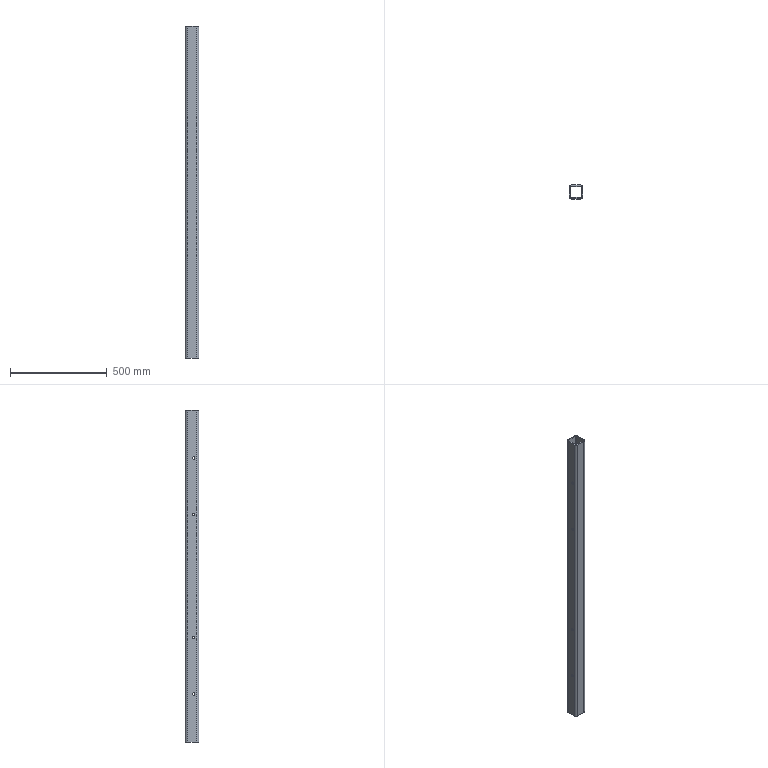Part | SolidWorks | features Extrusion 1, ICE 1, LPattern 1 | 1 solid | 34 faces | box 70 x 70 x 1716 mm | volume 2470318 mm3 | cylinder 24 | plane 10 | commonest cylinder face diameters 13 x16 12 x4 24 x4
STEP:
#1=CARTESIAN_POINT('',(70.,26.,1461.5));
#2=VERTEX_POINT('',#1);
#3=CARTESIAN_POINT('',(70.,26.,1474.5));
#4=VERTEX_POINT('',#3);
#5=CARTESIAN_POINT('',(70.,26.,1468.));
#6=DIRECTION('',(-1.,0.,0.));
#7=DIRECTION('',(0.,0.,1.));
#8=AXIS2_PLACEMENT_3D('',#5,#6,#7);
#9=CIRCLE('',#8,6.5);
#10=EDGE_CURVE('',#2,#4,#9,.T.);
#11=ORIENTED_EDGE('',*,*,#10,.F.);
#12=CARTESIAN_POINT('',(64.,26.,1461.5));
#13=VERTEX_POINT('',#12);
#14=CARTESIAN_POINT('',(70.,26.,1461.5));
#15=DIRECTION('',(-1.,0.,0.));
#16=VECTOR('',#15,1000.);
#17=LINE('',#14,#16);
#18=EDGE_CURVE('',#2,#13,#17,.T.);
#19=ORIENTED_EDGE('',*,*,#18,.T.);
#20=CARTESIAN_POINT('',(64.,26.,1474.5));
#21=VERTEX_POINT('',#20);
#22=CARTESIAN_POINT('',(64.,26.,1468.));
#23=DIRECTION('',(-1.,0.,0.));
#24=DIRECTION('',(0.,0.,1.));
#25=AXIS2_PLACEMENT_3D('',#22,#23,#24);
#26=CIRCLE('',#25,6.5);
#27=EDGE_CURVE('',#13,#21,#26,.T.);
#28=ORIENTED_EDGE('',*,*,#27,.T.);
#29=CARTESIAN_POINT('',(70.,26.,1474.5));
#30=DIRECTION('',(-1.,0.,0.));
#31=VECTOR('',#30,1000.);
#32=LINE('',#29,#31);
#33=EDGE_CURVE('',#4,#21,#32,.T.);
#34=ORIENTED_EDGE('',*,*,#33,.F.);
#35=EDGE_LOOP('',(#11,#19,#28,#34));
#36=FACE_OUTER_BOUND('',#35,.T.);
#37=CARTESIAN_POINT('',(70.,26.,1468.));
#38=DIRECTION('',(-1.,0.,0.));
#39=DIRECTION('',(0.,0.,1.));
#40=AXIS2_PLACEMENT_3D('',#37,#38,#39);
#41=CYLINDRICAL_SURFACE('',#40,6.5);
#42=ADVANCED_FACE('',(#36),#41,.F.);
#43=CARTESIAN_POINT('',(6.,26.,1474.5));
#44=VERTEX_POINT('',#43);
#45=CARTESIAN_POINT('',(6.,26.,1461.5));
#46=VERTEX_POINT('',#45);
#47=CARTESIAN_POINT('',(6.,26.,1468.));
#48=DIRECTION('',(1.,0.,0.));
#49=DIRECTION('',(0.,0.,-1.));
#50=AXIS2_PLACEMENT_3D('',#47,#48,#49);
#51=CIRCLE('',#50,6.5);
#52=EDGE_CURVE('',#44,#46,#51,.T.);
#53=ORIENTED_EDGE('',*,*,#52,.T.);
#54=CARTESIAN_POINT('',(0.,26.,1461.5));
#55=VERTEX_POINT('',#54);
#56=CARTESIAN_POINT('',(70.,26.,1461.5));
#57=DIRECTION('',(-1.,0.,0.));
#58=VECTOR('',#57,1000.);
#59=LINE('',#56,#58);
#60=EDGE_CURVE('',#46,#55,#59,.T.);
#61=ORIENTED_EDGE('',*,*,#60,.T.);
#62=CARTESIAN_POINT('',(0.,26.,1474.5));
#63=VERTEX_POINT('',#62);
#64=CARTESIAN_POINT('',(0.,26.,1468.));
#65=DIRECTION('',(-1.,0.,0.));
#66=DIRECTION('',(0.,0.,1.));
#67=AXIS2_PLACEMENT_3D('',#64,#65,#66);
#68=CIRCLE('',#67,6.5);
#69=EDGE_CURVE('',#55,#63,#68,.T.);
#70=ORIENTED_EDGE('',*,*,#69,.T.);
#71=CARTESIAN_POINT('',(70.,26.,1474.5));
#72=DIRECTION('',(-1.,0.,0.));
#73=VECTOR('',#72,1000.);
#74=LINE('',#71,#73);
#75=EDGE_CURVE('',#44,#63,#74,.T.);
#76=ORIENTED_EDGE('',*,*,#75,.F.);
#77=EDGE_LOOP('',(#53,#61,#70,#76));
#78=FACE_OUTER_BOUND('',#77,.T.);
#79=CARTESIAN_POINT('',(70.,26.,1468.));
#80=DIRECTION('',(-1.,0.,0.));
#81=DIRECTION('',(0.,0.,1.));
#82=AXIS2_PLACEMENT_3D('',#79,#80,#81);
#83=CYLINDRICAL_SURFACE('',#82,6.5);
#84=ADVANCED_FACE('',(#78),#83,.F.);
#85=CARTESIAN_POINT('',(70.,26.,1169.5));
#86=VERTEX_POINT('',#85);
#87=CARTESIAN_POINT('',(70.,26.,1182.5));
#88=VERTEX_POINT('',#87);
#89=CARTESIAN_POINT('',(70.,26.,1176.));
#90=DIRECTION('',(-1.,0.,0.));
#91=DIRECTION('',(0.,0.,1.));
#92=AXIS2_PLACEMENT_3D('',#89,#90,#91);
#93=CIRCLE('',#92,6.5);
#94=EDGE_CURVE('',#86,#88,#93,.T.);
#95=ORIENTED_EDGE('',*,*,#94,.F.);
#96=CARTESIAN_POINT('',(64.,26.,1169.5));
#97=VERTEX_POINT('',#96);
#98=CARTESIAN_POINT('',(70.,26.,1169.5));
#99=DIRECTION('',(-1.,0.,0.));
#100=VECTOR('',#99,1000.);
#101=LINE('',#98,#100);
#102=EDGE_CURVE('',#86,#97,#101,.T.);
#103=ORIENTED_EDGE('',*,*,#102,.T.);
#104=CARTESIAN_POINT('',(64.,26.,1182.5));
#105=VERTEX_POINT('',#104);
#106=CARTESIAN_POINT('',(64.,26.,1176.));
#107=DIRECTION('',(-1.,0.,0.));
#108=DIRECTION('',(0.,0.,1.));
#109=AXIS2_PLACEMENT_3D('',#106,#107,#108);
#110=CIRCLE('',#109,6.5);
#111=EDGE_CURVE('',#97,#105,#110,.T.);
#112=ORIENTED_EDGE('',*,*,#111,.T.);
#113=CARTESIAN_POINT('',(70.,26.,1182.5));
#114=DIRECTION('',(-1.,0.,0.));
#115=VECTOR('',#114,1000.);
#116=LINE('',#113,#115);
#117=EDGE_CURVE('',#88,#105,#116,.T.);
#118=ORIENTED_EDGE('',*,*,#117,.F.);
#119=EDGE_LOOP('',(#95,#103,#112,#118));
#120=FACE_OUTER_BOUND('',#119,.T.);
#121=CARTESIAN_POINT('',(70.,26.,1176.));
#122=DIRECTION('',(-1.,0.,0.));
#123=DIRECTION('',(0.,0.,1.));
#124=AXIS2_PLACEMENT_3D('',#121,#122,#123);
#125=CYLINDRICAL_SURFACE('',#124,6.5);
#126=ADVANCED_FACE('',(#120),#125,.F.);
#127=CARTESIAN_POINT('',(6.,26.,1182.5));
#128=VERTEX_POINT('',#127);
#129=CARTESIAN_POINT('',(6.,26.,1169.5));
#130=VERTEX_POINT('',#129);
#131=CARTESIAN_POINT('',(6.,26.,1176.));
#132=DIRECTION('',(1.,0.,0.));
#133=DIRECTION('',(0.,0.,-1.));
#134=AXIS2_PLACEMENT_3D('',#131,#132,#133);
#135=CIRCLE('',#134,6.5);
#136=EDGE_CURVE('',#128,#130,#135,.T.);
#137=ORIENTED_EDGE('',*,*,#136,.T.);
#138=CARTESIAN_POINT('',(0.,26.,1169.5));
#139=VERTEX_POINT('',#138);
#140=CARTESIAN_POINT('',(70.,26.,1169.5));
#141=DIRECTION('',(-1.,0.,0.));
#142=VECTOR('',#141,1000.);
#143=LINE('',#140,#142);
#144=EDGE_CURVE('',#130,#139,#143,.T.);
#145=ORIENTED_EDGE('',*,*,#144,.T.);
#146=CARTESIAN_POINT('',(0.,26.,1182.5));
#147=VERTEX_POINT('',#146);
#148=CARTESIAN_POINT('',(0.,26.,1176.));
#149=DIRECTION('',(-1.,0.,0.));
#150=DIRECTION('',(0.,0.,1.));
#151=AXIS2_PLACEMENT_3D('',#148,#149,#150);
#152=CIRCLE('',#151,6.5);
#153=EDGE_CURVE('',#139,#147,#152,.T.);
#154=ORIENTED_EDGE('',*,*,#153,.T.);
#155=CARTESIAN_POINT('',(70.,26.,1182.5));
#156=DIRECTION('',(-1.,0.,0.));
#157=VECTOR('',#156,1000.);
#158=LINE('',#155,#157);
#159=EDGE_CURVE('',#128,#147,#158,.T.);
#160=ORIENTED_EDGE('',*,*,#159,.F.);
#161=EDGE_LOOP('',(#137,#145,#154,#160));
#162=FACE_OUTER_BOUND('',#161,.T.);
#163=CARTESIAN_POINT('',(70.,26.,1176.));
#164=DIRECTION('',(-1.,0.,0.));
#165=DIRECTION('',(0.,0.,1.));
#166=AXIS2_PLACEMENT_3D('',#163,#164,#165);
#167=CYLINDRICAL_SURFACE('',#166,6.5);
#168=ADVANCED_FACE('',(#162),#167,.F.);
#169=CARTESIAN_POINT('',(70.,26.,533.5));
#170=VERTEX_POINT('',#169);
#171=CARTESIAN_POINT('',(70.,26.,546.5));
#172=VERTEX_POINT('',#171);
#173=CARTESIAN_POINT('',(70.,26.,540.));
#174=DIRECTION('',(-1.,0.,0.));
#175=DIRECTION('',(0.,0.,1.));
#176=AXIS2_PLACEMENT_3D('',#173,#174,#175);
#177=CIRCLE('',#176,6.5);
#178=EDGE_CURVE('',#170,#172,#177,.T.);
#179=ORIENTED_EDGE('',*,*,#178,.F.);
#180=CARTESIAN_POINT('',(64.,26.,533.5));
#181=VERTEX_POINT('',#180);
#182=CARTESIAN_POINT('',(70.,26.,533.5));
#183=DIRECTION('',(-1.,0.,0.));
#184=VECTOR('',#183,1000.);
#185=LINE('',#182,#184);
#186=EDGE_CURVE('',#170,#181,#185,.T.);
#187=ORIENTED_EDGE('',*,*,#186,.T.);
#188=CARTESIAN_POINT('',(64.,26.,546.5));
#189=VERTEX_POINT('',#188);
#190=CARTESIAN_POINT('',(64.,26.,540.));
#191=DIRECTION('',(-1.,0.,0.));
#192=DIRECTION('',(0.,0.,1.));
#193=AXIS2_PLACEMENT_3D('',#190,#191,#192);
#194=CIRCLE('',#193,6.5);
#195=EDGE_CURVE('',#181,#189,#194,.T.);
#196=ORIENTED_EDGE('',*,*,#195,.T.);
#197=CARTESIAN_POINT('',(70.,26.,546.5));
#198=DIRECTION('',(-1.,0.,0.));
#199=VECTOR('',#198,1000.);
#200=LINE('',#197,#199);
#201=EDGE_CURVE('',#172,#189,#200,.T.);
#202=ORIENTED_EDGE('',*,*,#201,.F.);
#203=EDGE_LOOP('',(#179,#187,#196,#202));
#204=FACE_OUTER_BOUND('',#203,.T.);
#205=CARTESIAN_POINT('',(70.,26.,540.));
#206=DIRECTION('',(-1.,0.,0.));
#207=DIRECTION('',(0.,0.,1.));
#208=AXIS2_PLACEMENT_3D('',#205,#206,#207);
#209=CYLINDRICAL_SURFACE('',#208,6.5);
#210=ADVANCED_FACE('',(#204),#209,.F.);
#211=CARTESIAN_POINT('',(6.,26.,546.5));
#212=VERTEX_POINT('',#211);
#213=CARTESIAN_POINT('',(6.,26.,533.5));
#214=VERTEX_POINT('',#213);
#215=CARTESIAN_POINT('',(6.,26.,540.));
#216=DIRECTION('',(1.,0.,0.));
#217=DIRECTION('',(0.,0.,-1.));
#218=AXIS2_PLACEMENT_3D('',#215,#216,#217);
#219=CIRCLE('',#218,6.5);
#220=EDGE_CURVE('',#212,#214,#219,.T.);
#221=ORIENTED_EDGE('',*,*,#220,.T.);
#222=CARTESIAN_POINT('',(0.,26.,533.5));
#223=VERTEX_POINT('',#222);
#224=CARTESIAN_POINT('',(70.,26.,533.5));
#225=DIRECTION('',(-1.,0.,0.));
#226=VECTOR('',#225,1000.);
#227=LINE('',#224,#226);
#228=EDGE_CURVE('',#214,#223,#227,.T.);
#229=ORIENTED_EDGE('',*,*,#228,.T.);
#230=CARTESIAN_POINT('',(0.,26.,546.5));
#231=VERTEX_POINT('',#230);
#232=CARTESIAN_POINT('',(0.,26.,540.));
#233=DIRECTION('',(-1.,0.,0.));
#234=DIRECTION('',(0.,0.,1.));
#235=AXIS2_PLACEMENT_3D('',#232,#233,#234);
#236=CIRCLE('',#235,6.5);
#237=EDGE_CURVE('',#223,#231,#236,.T.);
#238=ORIENTED_EDGE('',*,*,#237,.T.);
#239=CARTESIAN_POINT('',(70.,26.,546.5));
#240=DIRECTION('',(-1.,0.,0.));
#241=VECTOR('',#240,1000.);
#242=LINE('',#239,#241);
#243=EDGE_CURVE('',#212,#231,#242,.T.);
#244=ORIENTED_EDGE('',*,*,#243,.F.);
#245=EDGE_LOOP('',(#221,#229,#238,#244));
#246=FACE_OUTER_BOUND('',#245,.T.);
#247=CARTESIAN_POINT('',(70.,26.,540.));
#248=DIRECTION('',(-1.,0.,0.));
#249=DIRECTION('',(0.,0.,1.));
#250=AXIS2_PLACEMENT_3D('',#247,#248,#249);
#251=CYLINDRICAL_SURFACE('',#250,6.5);
#252=ADVANCED_FACE('',(#246),#251,.F.);
#253=CARTESIAN_POINT('',(70.,26.,241.5));
#254=VERTEX_POINT('',#253);
#255=CARTESIAN_POINT('',(70.,26.,254.5));
#256=VERTEX_POINT('',#255);
#257=CARTESIAN_POINT('',(70.,26.,248.));
#258=DIRECTION('',(-1.,0.,0.));
#259=DIRECTION('',(0.,0.,1.));
#260=AXIS2_PLACEMENT_3D('',#257,#258,#259);
#261=CIRCLE('',#260,6.5);
#262=EDGE_CURVE('',#254,#256,#261,.T.);
#263=ORIENTED_EDGE('',*,*,#262,.F.);
#264=CARTESIAN_POINT('',(64.,26.,241.5));
#265=VERTEX_POINT('',#264);
#266=CARTESIAN_POINT('',(70.,26.,241.5));
#267=DIRECTION('',(-1.,0.,0.));
#268=VECTOR('',#267,1000.);
#269=LINE('',#266,#268);
#270=EDGE_CURVE('',#254,#265,#269,.T.);
#271=ORIENTED_EDGE('',*,*,#270,.T.);
#272=CARTESIAN_POINT('',(64.,26.,254.5));
#273=VERTEX_POINT('',#272);
#274=CARTESIAN_POINT('',(64.,26.,248.));
#275=DIRECTION('',(-1.,0.,0.));
#276=DIRECTION('',(0.,0.,1.));
#277=AXIS2_PLACEMENT_3D('',#274,#275,#276);
#278=CIRCLE('',#277,6.5);
#279=EDGE_CURVE('',#265,#273,#278,.T.);
#280=ORIENTED_EDGE('',*,*,#279,.T.);
#281=CARTESIAN_POINT('',(70.,26.,254.5));
#282=DIRECTION('',(-1.,0.,0.));
#283=VECTOR('',#282,1000.);
#284=LINE('',#281,#283);
#285=EDGE_CURVE('',#256,#273,#284,.T.);
#286=ORIENTED_EDGE('',*,*,#285,.F.);
#287=EDGE_LOOP('',(#263,#271,#280,#286));
#288=FACE_OUTER_BOUND('',#287,.T.);
#289=CARTESIAN_POINT('',(70.,26.,248.));
#290=DIRECTION('',(-1.,0.,0.));
#291=DIRECTION('',(0.,0.,1.));
#292=AXIS2_PLACEMENT_3D('',#289,#290,#291);
#293=CYLINDRICAL_SURFACE('',#292,6.5);
#294=ADVANCED_FACE('',(#288),#293,.F.);
#295=CARTESIAN_POINT('',(6.,26.,254.5));
#296=VERTEX_POINT('',#295);
#297=CARTESIAN_POINT('',(6.,26.,241.5));
#298=VERTEX_POINT('',#297);
#299=CARTESIAN_POINT('',(6.,26.,248.));
#300=DIRECTION('',(1.,0.,0.));
#301=DIRECTION('',(0.,0.,-1.));
#302=AXIS2_PLACEMENT_3D('',#299,#300,#301);
#303=CIRCLE('',#302,6.5);
#304=EDGE_CURVE('',#296,#298,#303,.T.);
#305=ORIENTED_EDGE('',*,*,#304,.T.);
#306=CARTESIAN_POINT('',(0.,26.,241.5));
#307=VERTEX_POINT('',#306);
#308=CARTESIAN_POINT('',(70.,26.,241.5));
#309=DIRECTION('',(-1.,0.,0.));
#310=VECTOR('',#309,1000.);
#311=LINE('',#308,#310);
#312=EDGE_CURVE('',#298,#307,#311,.T.);
#313=ORIENTED_EDGE('',*,*,#312,.T.);
#314=CARTESIAN_POINT('',(0.,26.,254.5));
#315=VERTEX_POINT('',#314);
#316=CARTESIAN_POINT('',(0.,26.,248.));
#317=DIRECTION('',(-1.,0.,0.));
#318=DIRECTION('',(0.,0.,1.));
#319=AXIS2_PLACEMENT_3D('',#316,#317,#318);
#320=CIRCLE('',#319,6.5);
#321=EDGE_CURVE('',#307,#315,#320,.T.);
#322=ORIENTED_EDGE('',*,*,#321,.T.);
#323=CARTESIAN_POINT('',(70.,26.,254.5));
#324=DIRECTION('',(-1.,0.,0.));
#325=VECTOR('',#324,1000.);
#326=LINE('',#323,#325);
#327=EDGE_CURVE('',#296,#315,#326,.T.);
#328=ORIENTED_EDGE('',*,*,#327,.F.);
#329=EDGE_LOOP('',(#305,#313,#322,#328));
#330=FACE_OUTER_BOUND('',#329,.T.);
#331=CARTESIAN_POINT('',(70.,26.,248.));
#332=DIRECTION('',(-1.,0.,0.));
#333=DIRECTION('',(0.,0.,1.));
#334=AXIS2_PLACEMENT_3D('',#331,#332,#333);
#335=CYLINDRICAL_SURFACE('',#334,6.5);
#336=ADVANCED_FACE('',(#330),#335,.F.);
#337=CARTESIAN_POINT('',(0.,12.,1716.));
#338=VERTEX_POINT('',#337);
#339=CARTESIAN_POINT('',(12.,0.,1716.));
#340=VERTEX_POINT('',#339);
#341=CARTESIAN_POINT('',(12.,12.,1716.));
#342=DIRECTION('',(0.,0.,1.));
#343=DIRECTION('',(-1.,0.,0.));
#344=AXIS2_PLACEMENT_3D('',#341,#342,#343);
#345=CIRCLE('',#344,12.);
#346=EDGE_CURVE('',#338,#340,#345,.T.);
#347=ORIENTED_EDGE('',*,*,#346,.T.);
#348=CARTESIAN_POINT('',(58.,0.,1716.));
#349=VERTEX_POINT('',#348);
#350=CARTESIAN_POINT('',(12.,0.,1716.));
#351=DIRECTION('',(1.,0.,0.));
#352=VECTOR('',#351,1000.);
#353=LINE('',#350,#352);
#354=EDGE_CURVE('',#340,#349,#353,.T.);
#355=ORIENTED_EDGE('',*,*,#354,.T.);
#356=CARTESIAN_POINT('',(70.,12.,1716.));
#357=VERTEX_POINT('',#356);
#358=CARTESIAN_POINT('',(58.,12.,1716.));
#359=DIRECTION('',(0.,0.,1.));
#360=DIRECTION('',(1.,0.,0.));
#361=AXIS2_PLACEMENT_3D('',#358,#359,#360);
#362=CIRCLE('',#361,12.);
#363=EDGE_CURVE('',#349,#357,#362,.T.);
#364=ORIENTED_EDGE('',*,*,#363,.T.);
#365=CARTESIAN_POINT('',(70.,58.,1716.));
#366=VERTEX_POINT('',#365);
#367=CARTESIAN_POINT('',(70.,12.,1716.));
#368=DIRECTION('',(0.,1.,0.));
#369=VECTOR('',#368,1000.);
#370=LINE('',#367,#369);
#371=EDGE_CURVE('',#357,#366,#370,.T.);
#372=ORIENTED_EDGE('',*,*,#371,.T.);
#373=CARTESIAN_POINT('',(58.,70.,1716.));
#374=VERTEX_POINT('',#373);
#375=CARTESIAN_POINT('',(58.,58.,1716.));
#376=DIRECTION('',(0.,0.,1.));
#377=DIRECTION('',(-1.,0.,0.));
#378=AXIS2_PLACEMENT_3D('',#375,#376,#377);
#379=CIRCLE('',#378,12.);
#380=EDGE_CURVE('',#366,#374,#379,.T.);
#381=ORIENTED_EDGE('',*,*,#380,.T.);
#382=CARTESIAN_POINT('',(12.,70.,1716.));
#383=VERTEX_POINT('',#382);
#384=CARTESIAN_POINT('',(12.,70.,1716.));
#385=DIRECTION('',(-1.,0.,0.));
#386=VECTOR('',#385,1000.);
#387=LINE('',#384,#386);
#388=EDGE_CURVE('',#374,#383,#387,.T.);
#389=ORIENTED_EDGE('',*,*,#388,.T.);
#390=CARTESIAN_POINT('',(0.,58.,1716.));
#391=VERTEX_POINT('',#390);
#392=CARTESIAN_POINT('',(12.,58.,1716.));
#393=DIRECTION('',(0.,0.,1.));
#394=DIRECTION('',(-1.,0.,0.));
#395=AXIS2_PLACEMENT_3D('',#392,#393,#394);
#396=CIRCLE('',#395,12.);
#397=EDGE_CURVE('',#383,#391,#396,.T.);
#398=ORIENTED_EDGE('',*,*,#397,.T.);
#399=CARTESIAN_POINT('',(0.,12.,1716.));
#400=DIRECTION('',(0.,-1.,0.));
#401=VECTOR('',#400,1000.);
#402=LINE('',#399,#401);
#403=EDGE_CURVE('',#391,#338,#402,.T.);
#404=ORIENTED_EDGE('',*,*,#403,.T.);
#405=EDGE_LOOP('',(#347,#355,#364,#372,#381,#389,#398,#404));
#406=FACE_OUTER_BOUND('',#405,.T.);
#407=CARTESIAN_POINT('',(6.,12.,1716.));
#408=VERTEX_POINT('',#407);
#409=CARTESIAN_POINT('',(12.,6.,1716.));
#410=VERTEX_POINT('',#409);
#411=CARTESIAN_POINT('',(12.,12.,1716.));
#412=DIRECTION('',(0.,0.,1.));
#413=DIRECTION('',(-1.,0.,0.));
#414=AXIS2_PLACEMENT_3D('',#411,#412,#413);
#415=CIRCLE('',#414,6.);
#416=EDGE_CURVE('',#408,#410,#415,.T.);
#417=ORIENTED_EDGE('',*,*,#416,.F.);
#418=CARTESIAN_POINT('',(6.,58.,1716.));
#419=VERTEX_POINT('',#418);
#420=CARTESIAN_POINT('',(6.,12.,1716.));
#421=DIRECTION('',(0.,-1.,0.));
#422=VECTOR('',#421,1000.);
#423=LINE('',#420,#422);
#424=EDGE_CURVE('',#419,#408,#423,.T.);
#425=ORIENTED_EDGE('',*,*,#424,.F.);
#426=CARTESIAN_POINT('',(12.,64.,1716.));
#427=VERTEX_POINT('',#426);
#428=CARTESIAN_POINT('',(12.,58.,1716.));
#429=DIRECTION('',(0.,0.,1.));
#430=DIRECTION('',(-1.,0.,0.));
#431=AXIS2_PLACEMENT_3D('',#428,#429,#430);
#432=CIRCLE('',#431,6.);
#433=EDGE_CURVE('',#427,#419,#432,.T.);
#434=ORIENTED_EDGE('',*,*,#433,.F.);
#435=CARTESIAN_POINT('',(58.,64.,1716.));
#436=VERTEX_POINT('',#435);
#437=CARTESIAN_POINT('',(12.,64.,1716.));
#438=DIRECTION('',(-1.,0.,0.));
#439=VECTOR('',#438,1000.);
#440=LINE('',#437,#439);
#441=EDGE_CURVE('',#436,#427,#440,.T.);
#442=ORIENTED_EDGE('',*,*,#441,.F.);
#443=CARTESIAN_POINT('',(64.,58.,1716.));
#444=VERTEX_POINT('',#443);
#445=CARTESIAN_POINT('',(58.,58.,1716.));
#446=DIRECTION('',(0.,0.,1.));
#447=DIRECTION('',(-1.,0.,0.));
#448=AXIS2_PLACEMENT_3D('',#445,#446,#447);
#449=CIRCLE('',#448,6.);
#450=EDGE_CURVE('',#444,#436,#449,.T.);
#451=ORIENTED_EDGE('',*,*,#450,.F.);
#452=CARTESIAN_POINT('',(64.,12.,1716.));
#453=VERTEX_POINT('',#452);
#454=CARTESIAN_POINT('',(64.,12.,1716.));
#455=DIRECTION('',(0.,1.,0.));
#456=VECTOR('',#455,1000.);
#457=LINE('',#454,#456);
#458=EDGE_CURVE('',#453,#444,#457,.T.);
#459=ORIENTED_EDGE('',*,*,#458,.F.);
#460=CARTESIAN_POINT('',(58.,6.,1716.));
#461=VERTEX_POINT('',#460);
#462=CARTESIAN_POINT('',(58.,12.,1716.));
#463=DIRECTION('',(0.,0.,1.));
#464=DIRECTION('',(1.,0.,0.));
#465=AXIS2_PLACEMENT_3D('',#462,#463,#464);
#466=CIRCLE('',#465,6.);
#467=EDGE_CURVE('',#461,#453,#466,.T.);
#468=ORIENTED_EDGE('',*,*,#467,.F.);
#469=CARTESIAN_POINT('',(12.,6.,1716.));
#470=DIRECTION('',(1.,0.,0.));
#471=VECTOR('',#470,1000.);
#472=LINE('',#469,#471);
#473=EDGE_CURVE('',#410,#461,#472,.T.);
#474=ORIENTED_EDGE('',*,*,#473,.F.);
#475=EDGE_LOOP('',(#417,#425,#434,#442,#451,#459,#468,#474));
#476=FACE_BOUND('',#475,.T.);
#477=CARTESIAN_POINT('',(12.,12.,1716.));
#478=DIRECTION('',(0.,0.,-1.));
#479=DIRECTION('',(-1.,0.,0.));
#480=AXIS2_PLACEMENT_3D('',#477,#478,#479);
#481=PLANE('',#480);
#482=ADVANCED_FACE('',(#406,#476),#481,.F.);
#483=CARTESIAN_POINT('',(0.,12.,0.));
#484=VERTEX_POINT('',#483);
#485=CARTESIAN_POINT('',(12.,0.,0.));
#486=VERTEX_POINT('',#485);
#487=CARTESIAN_POINT('',(12.,12.,0.));
#488=DIRECTION('',(0.,0.,1.));
#489=DIRECTION('',(-1.,0.,0.));
#490=AXIS2_PLACEMENT_3D('',#487,#488,#489);
#491=CIRCLE('',#490,12.);
#492=EDGE_CURVE('',#484,#486,#491,.T.);
#493=ORIENTED_EDGE('',*,*,#492,.F.);
#494=CARTESIAN_POINT('',(0.,58.,0.));
#495=VERTEX_POINT('',#494);
#496=CARTESIAN_POINT('',(0.,12.,0.));
#497=DIRECTION('',(0.,-1.,0.));
#498=VECTOR('',#497,1000.);
#499=LINE('',#496,#498);
#500=EDGE_CURVE('',#495,#484,#499,.T.);
#501=ORIENTED_EDGE('',*,*,#500,.F.);
#502=CARTESIAN_POINT('',(12.,70.,0.));
#503=VERTEX_POINT('',#502);
#504=CARTESIAN_POINT('',(12.,58.,0.));
#505=DIRECTION('',(0.,0.,1.));
#506=DIRECTION('',(-1.,0.,0.));
#507=AXIS2_PLACEMENT_3D('',#504,#505,#506);
#508=CIRCLE('',#507,12.);
#509=EDGE_CURVE('',#503,#495,#508,.T.);
#510=ORIENTED_EDGE('',*,*,#509,.F.);
#511=CARTESIAN_POINT('',(58.,70.,0.));
#512=VERTEX_POINT('',#511);
#513=CARTESIAN_POINT('',(12.,70.,0.));
#514=DIRECTION('',(-1.,0.,0.));
#515=VECTOR('',#514,1000.);
#516=LINE('',#513,#515);
#517=EDGE_CURVE('',#512,#503,#516,.T.);
#518=ORIENTED_EDGE('',*,*,#517,.F.);
#519=CARTESIAN_POINT('',(70.,58.,0.));
#520=VERTEX_POINT('',#519);
#521=CARTESIAN_POINT('',(58.,58.,0.));
#522=DIRECTION('',(0.,0.,1.));
#523=DIRECTION('',(-1.,0.,0.));
#524=AXIS2_PLACEMENT_3D('',#521,#522,#523);
#525=CIRCLE('',#524,12.);
#526=EDGE_CURVE('',#520,#512,#525,.T.);
#527=ORIENTED_EDGE('',*,*,#526,.F.);
#528=CARTESIAN_POINT('',(70.,12.,0.));
#529=VERTEX_POINT('',#528);
#530=CARTESIAN_POINT('',(70.,12.,0.));
#531=DIRECTION('',(0.,1.,0.));
#532=VECTOR('',#531,1000.);
#533=LINE('',#530,#532);
#534=EDGE_CURVE('',#529,#520,#533,.T.);
#535=ORIENTED_EDGE('',*,*,#534,.F.);
#536=CARTESIAN_POINT('',(58.,0.,0.));
#537=VERTEX_POINT('',#536);
#538=CARTESIAN_POINT('',(58.,12.,0.));
#539=DIRECTION('',(0.,0.,1.));
#540=DIRECTION('',(1.,0.,0.));
#541=AXIS2_PLACEMENT_3D('',#538,#539,#540);
#542=CIRCLE('',#541,12.);
#543=EDGE_CURVE('',#537,#529,#542,.T.);
#544=ORIENTED_EDGE('',*,*,#543,.F.);
#545=CARTESIAN_POINT('',(12.,0.,0.));
#546=DIRECTION('',(1.,0.,0.));
#547=VECTOR('',#546,1000.);
#548=LINE('',#545,#547);
#549=EDGE_CURVE('',#486,#537,#548,.T.);
#550=ORIENTED_EDGE('',*,*,#549,.F.);
#551=EDGE_LOOP('',(#493,#501,#510,#518,#527,#535,#544,#550));
#552=FACE_OUTER_BOUND('',#551,.T.);
#553=CARTESIAN_POINT('',(6.,58.,0.));
#554=VERTEX_POINT('',#553);
#555=CARTESIAN_POINT('',(6.,12.,0.));
#556=VERTEX_POINT('',#555);
#557=CARTESIAN_POINT('',(6.,12.,0.));
#558=DIRECTION('',(0.,-1.,0.));
#559=VECTOR('',#558,1000.);
#560=LINE('',#557,#559);
#561=EDGE_CURVE('',#554,#556,#560,.T.);
#562=ORIENTED_EDGE('',*,*,#561,.T.);
#563=CARTESIAN_POINT('',(12.,6.,0.));
#564=VERTEX_POINT('',#563);
#565=CARTESIAN_POINT('',(12.,12.,0.));
#566=DIRECTION('',(0.,0.,1.));
#567=DIRECTION('',(-1.,0.,0.));
#568=AXIS2_PLACEMENT_3D('',#565,#566,#567);
#569=CIRCLE('',#568,6.);
#570=EDGE_CURVE('',#556,#564,#569,.T.);
#571=ORIENTED_EDGE('',*,*,#570,.T.);
#572=CARTESIAN_POINT('',(58.,6.,0.));
#573=VERTEX_POINT('',#572);
#574=CARTESIAN_POINT('',(12.,6.,0.));
#575=DIRECTION('',(1.,0.,0.));
#576=VECTOR('',#575,1000.);
#577=LINE('',#574,#576);
#578=EDGE_CURVE('',#564,#573,#577,.T.);
#579=ORIENTED_EDGE('',*,*,#578,.T.);
#580=CARTESIAN_POINT('',(64.,12.,0.));
#581=VERTEX_POINT('',#580);
#582=CARTESIAN_POINT('',(58.,12.,0.));
#583=DIRECTION('',(0.,0.,1.));
#584=DIRECTION('',(1.,0.,0.));
#585=AXIS2_PLACEMENT_3D('',#582,#583,#584);
#586=CIRCLE('',#585,6.);
#587=EDGE_CURVE('',#573,#581,#586,.T.);
#588=ORIENTED_EDGE('',*,*,#587,.T.);
#589=CARTESIAN_POINT('',(64.,58.,0.));
#590=VERTEX_POINT('',#589);
#591=CARTESIAN_POINT('',(64.,12.,0.));
#592=DIRECTION('',(0.,1.,0.));
#593=VECTOR('',#592,1000.);
#594=LINE('',#591,#593);
#595=EDGE_CURVE('',#581,#590,#594,.T.);
#596=ORIENTED_EDGE('',*,*,#595,.T.);
#597=CARTESIAN_POINT('',(58.,64.,0.));
#598=VERTEX_POINT('',#597);
#599=CARTESIAN_POINT('',(58.,58.,0.));
#600=DIRECTION('',(0.,0.,1.));
#601=DIRECTION('',(-1.,0.,0.));
#602=AXIS2_PLACEMENT_3D('',#599,#600,#601);
#603=CIRCLE('',#602,6.);
#604=EDGE_CURVE('',#590,#598,#603,.T.);
#605=ORIENTED_EDGE('',*,*,#604,.T.);
#606=CARTESIAN_POINT('',(12.,64.,0.));
#607=VERTEX_POINT('',#606);
#608=CARTESIAN_POINT('',(12.,64.,0.));
#609=DIRECTION('',(-1.,0.,0.));
#610=VECTOR('',#609,1000.);
#611=LINE('',#608,#610);
#612=EDGE_CURVE('',#598,#607,#611,.T.);
#613=ORIENTED_EDGE('',*,*,#612,.T.);
#614=CARTESIAN_POINT('',(12.,58.,0.));
#615=DIRECTION('',(0.,0.,1.));
#616=DIRECTION('',(-1.,0.,0.));
#617=AXIS2_PLACEMENT_3D('',#614,#615,#616);
#618=CIRCLE('',#617,6.);
#619=EDGE_CURVE('',#607,#554,#618,.T.);
#620=ORIENTED_EDGE('',*,*,#619,.T.);
#621=EDGE_LOOP('',(#562,#571,#579,#588,#596,#605,#613,#620));
#622=FACE_BOUND('',#621,.T.);
#623=CARTESIAN_POINT('',(12.,12.,0.));
#624=DIRECTION('',(0.,0.,-1.));
#625=DIRECTION('',(-1.,0.,0.));
#626=AXIS2_PLACEMENT_3D('',#623,#624,#625);
#627=PLANE('',#626);
#628=ADVANCED_FACE('',(#552,#622),#627,.T.);
#629=ORIENTED_EDGE('',*,*,#492,.T.);
#630=CARTESIAN_POINT('',(12.,0.,1716.));
#631=DIRECTION('',(0.,0.,-1.));
#632=VECTOR('',#631,1000.);
#633=LINE('',#630,#632);
#634=EDGE_CURVE('',#340,#486,#633,.T.);
#635=ORIENTED_EDGE('',*,*,#634,.F.);
#636=ORIENTED_EDGE('',*,*,#346,.F.);
#637=CARTESIAN_POINT('',(0.,12.,1716.));
#638=DIRECTION('',(0.,0.,-1.));
#639=VECTOR('',#638,1000.);
#640=LINE('',#637,#639);
#641=EDGE_CURVE('',#338,#484,#640,.T.);
#642=ORIENTED_EDGE('',*,*,#641,.T.);
#643=EDGE_LOOP('',(#629,#635,#636,#642));
#644=FACE_OUTER_BOUND('',#643,.T.);
#645=CARTESIAN_POINT('',(12.,12.,1716.));
#646=DIRECTION('',(0.,0.,-1.));
#647=DIRECTION('',(-1.,0.,0.));
#648=AXIS2_PLACEMENT_3D('',#645,#646,#647);
#649=CYLINDRICAL_SURFACE('',#648,12.);
#650=ADVANCED_FACE('',(#644),#649,.T.);
#651=ORIENTED_EDGE('',*,*,#549,.T.);
#652=CARTESIAN_POINT('',(58.,0.,1716.));
#653=DIRECTION('',(0.,0.,-1.));
#654=VECTOR('',#653,1000.);
#655=LINE('',#652,#654);
#656=EDGE_CURVE('',#349,#537,#655,.T.);
#657=ORIENTED_EDGE('',*,*,#656,.F.);
#658=ORIENTED_EDGE('',*,*,#354,.F.);
#659=ORIENTED_EDGE('',*,*,#634,.T.);
#660=EDGE_LOOP('',(#651,#657,#658,#659));
#661=FACE_OUTER_BOUND('',#660,.T.);
#662=CARTESIAN_POINT('',(12.,0.,1716.));
#663=DIRECTION('',(0.,1.,0.));
#664=DIRECTION('',(0.,0.,1.));
#665=AXIS2_PLACEMENT_3D('',#662,#663,#664);
#666=PLANE('',#665);
#667=ADVANCED_FACE('',(#661),#666,.F.);
#668=ORIENTED_EDGE('',*,*,#543,.T.);
#669=CARTESIAN_POINT('',(70.,12.,1716.));
#670=DIRECTION('',(0.,0.,-1.));
#671=VECTOR('',#670,1000.);
#672=LINE('',#669,#671);
#673=EDGE_CURVE('',#357,#529,#672,.T.);
#674=ORIENTED_EDGE('',*,*,#673,.F.);
#675=ORIENTED_EDGE('',*,*,#363,.F.);
#676=ORIENTED_EDGE('',*,*,#656,.T.);
#677=EDGE_LOOP('',(#668,#674,#675,#676));
#678=FACE_OUTER_BOUND('',#677,.T.);
#679=CARTESIAN_POINT('',(58.,12.,1716.));
#680=DIRECTION('',(0.,0.,-1.));
#681=DIRECTION('',(-1.,0.,0.));
#682=AXIS2_PLACEMENT_3D('',#679,#680,#681);
#683=CYLINDRICAL_SURFACE('',#682,12.);
#684=ADVANCED_FACE('',(#678),#683,.T.);
#685=CARTESIAN_POINT('',(70.,26.,1468.));
#686=DIRECTION('',(-1.,0.,0.));
#687=DIRECTION('',(0.,0.,1.));
#688=AXIS2_PLACEMENT_3D('',#685,#686,#687);
#689=CIRCLE('',#688,6.5);
#690=EDGE_CURVE('',#4,#2,#689,.T.);
#691=ORIENTED_EDGE('',*,*,#690,.T.);
#692=ORIENTED_EDGE('',*,*,#10,.T.);
#693=EDGE_LOOP('',(#691,#692));
#694=FACE_BOUND('',#693,.T.);
#695=CARTESIAN_POINT('',(70.,26.,1176.));
#696=DIRECTION('',(-1.,0.,0.));
#697=DIRECTION('',(0.,0.,1.));
#698=AXIS2_PLACEMENT_3D('',#695,#696,#697);
#699=CIRCLE('',#698,6.5);
#700=EDGE_CURVE('',#88,#86,#699,.T.);
#701=ORIENTED_EDGE('',*,*,#700,.T.);
#702=ORIENTED_EDGE('',*,*,#94,.T.);
#703=EDGE_LOOP('',(#701,#702));
#704=FACE_BOUND('',#703,.T.);
#705=CARTESIAN_POINT('',(70.,26.,540.));
#706=DIRECTION('',(-1.,0.,0.));
#707=DIRECTION('',(0.,0.,1.));
#708=AXIS2_PLACEMENT_3D('',#705,#706,#707);
#709=CIRCLE('',#708,6.5);
#710=EDGE_CURVE('',#172,#170,#709,.T.);
#711=ORIENTED_EDGE('',*,*,#710,.T.);
#712=ORIENTED_EDGE('',*,*,#178,.T.);
#713=EDGE_LOOP('',(#711,#712));
#714=FACE_BOUND('',#713,.T.);
#715=CARTESIAN_POINT('',(70.,26.,248.));
#716=DIRECTION('',(-1.,0.,0.));
#717=DIRECTION('',(0.,0.,1.));
#718=AXIS2_PLACEMENT_3D('',#715,#716,#717);
#719=CIRCLE('',#718,6.5);
#720=EDGE_CURVE('',#256,#254,#719,.T.);
#721=ORIENTED_EDGE('',*,*,#720,.T.);
#722=ORIENTED_EDGE('',*,*,#262,.T.);
#723=EDGE_LOOP('',(#721,#722));
#724=FACE_BOUND('',#723,.T.);
#725=ORIENTED_EDGE('',*,*,#534,.T.);
#726=CARTESIAN_POINT('',(70.,58.,1716.));
#727=DIRECTION('',(0.,0.,-1.));
#728=VECTOR('',#727,1000.);
#729=LINE('',#726,#728);
#730=EDGE_CURVE('',#366,#520,#729,.T.);
#731=ORIENTED_EDGE('',*,*,#730,.F.);
#732=ORIENTED_EDGE('',*,*,#371,.F.);
#733=ORIENTED_EDGE('',*,*,#673,.T.);
#734=EDGE_LOOP('',(#725,#731,#732,#733));
#735=FACE_OUTER_BOUND('',#734,.T.);
#736=CARTESIAN_POINT('',(70.,12.,1716.));
#737=DIRECTION('',(-1.,0.,0.));
#738=DIRECTION('',(0.,0.,1.));
#739=AXIS2_PLACEMENT_3D('',#736,#737,#738);
#740=PLANE('',#739);
#741=ADVANCED_FACE('',(#694,#704,#714,#724,#735),#740,.F.);
#742=ORIENTED_EDGE('',*,*,#526,.T.);
#743=CARTESIAN_POINT('',(58.,70.,1716.));
#744=DIRECTION('',(0.,0.,-1.));
#745=VECTOR('',#744,1000.);
#746=LINE('',#743,#745);
#747=EDGE_CURVE('',#374,#512,#746,.T.);
#748=ORIENTED_EDGE('',*,*,#747,.F.);
#749=ORIENTED_EDGE('',*,*,#380,.F.);
#750=ORIENTED_EDGE('',*,*,#730,.T.);
#751=EDGE_LOOP('',(#742,#748,#749,#750));
#752=FACE_OUTER_BOUND('',#751,.T.);
#753=CARTESIAN_POINT('',(58.,58.,1716.));
#754=DIRECTION('',(0.,0.,-1.));
#755=DIRECTION('',(-1.,0.,0.));
#756=AXIS2_PLACEMENT_3D('',#753,#754,#755);
#757=CYLINDRICAL_SURFACE('',#756,12.);
#758=ADVANCED_FACE('',(#752),#757,.T.);
#759=ORIENTED_EDGE('',*,*,#517,.T.);
#760=CARTESIAN_POINT('',(12.,70.,1716.));
#761=DIRECTION('',(0.,0.,-1.));
#762=VECTOR('',#761,1000.);
#763=LINE('',#760,#762);
#764=EDGE_CURVE('',#383,#503,#763,.T.);
#765=ORIENTED_EDGE('',*,*,#764,.F.);
#766=ORIENTED_EDGE('',*,*,#388,.F.);
#767=ORIENTED_EDGE('',*,*,#747,.T.);
#768=EDGE_LOOP('',(#759,#765,#766,#767));
#769=FACE_OUTER_BOUND('',#768,.T.);
#770=CARTESIAN_POINT('',(12.,70.,1716.));
#771=DIRECTION('',(0.,-1.,0.));
#772=DIRECTION('',(0.,0.,-1.));
#773=AXIS2_PLACEMENT_3D('',#770,#771,#772);
#774=PLANE('',#773);
#775=ADVANCED_FACE('',(#769),#774,.F.);
#776=ORIENTED_EDGE('',*,*,#509,.T.);
#777=CARTESIAN_POINT('',(0.,58.,1716.));
#778=DIRECTION('',(0.,0.,-1.));
#779=VECTOR('',#778,1000.);
#780=LINE('',#777,#779);
#781=EDGE_CURVE('',#391,#495,#780,.T.);
#782=ORIENTED_EDGE('',*,*,#781,.F.);
#783=ORIENTED_EDGE('',*,*,#397,.F.);
#784=ORIENTED_EDGE('',*,*,#764,.T.);
#785=EDGE_LOOP('',(#776,#782,#783,#784));
#786=FACE_OUTER_BOUND('',#785,.T.);
#787=CARTESIAN_POINT('',(12.,58.,1716.));
#788=DIRECTION('',(0.,0.,-1.));
#789=DIRECTION('',(-1.,0.,0.));
#790=AXIS2_PLACEMENT_3D('',#787,#788,#789);
#791=CYLINDRICAL_SURFACE('',#790,12.);
#792=ADVANCED_FACE('',(#786),#791,.T.);
#793=CARTESIAN_POINT('',(0.,26.,1468.));
#794=DIRECTION('',(-1.,0.,0.));
#795=DIRECTION('',(0.,0.,1.));
#796=AXIS2_PLACEMENT_3D('',#793,#794,#795);
#797=CIRCLE('',#796,6.5);
#798=EDGE_CURVE('',#63,#55,#797,.T.);
#799=ORIENTED_EDGE('',*,*,#798,.F.);
#800=ORIENTED_EDGE('',*,*,#69,.F.);
#801=EDGE_LOOP('',(#799,#800));
#802=FACE_BOUND('',#801,.T.);
#803=CARTESIAN_POINT('',(0.,26.,1176.));
#804=DIRECTION('',(-1.,0.,0.));
#805=DIRECTION('',(0.,0.,1.));
#806=AXIS2_PLACEMENT_3D('',#803,#804,#805);
#807=CIRCLE('',#806,6.5);
#808=EDGE_CURVE('',#147,#139,#807,.T.);
#809=ORIENTED_EDGE('',*,*,#808,.F.);
#810=ORIENTED_EDGE('',*,*,#153,.F.);
#811=EDGE_LOOP('',(#809,#810));
#812=FACE_BOUND('',#811,.T.);
#813=CARTESIAN_POINT('',(0.,26.,540.));
#814=DIRECTION('',(-1.,0.,0.));
#815=DIRECTION('',(0.,0.,1.));
#816=AXIS2_PLACEMENT_3D('',#813,#814,#815);
#817=CIRCLE('',#816,6.5);
#818=EDGE_CURVE('',#231,#223,#817,.T.);
#819=ORIENTED_EDGE('',*,*,#818,.F.);
#820=ORIENTED_EDGE('',*,*,#237,.F.);
#821=EDGE_LOOP('',(#819,#820));
#822=FACE_BOUND('',#821,.T.);
#823=CARTESIAN_POINT('',(0.,26.,248.));
#824=DIRECTION('',(-1.,0.,0.));
#825=DIRECTION('',(0.,0.,1.));
#826=AXIS2_PLACEMENT_3D('',#823,#824,#825);
#827=CIRCLE('',#826,6.5);
#828=EDGE_CURVE('',#315,#307,#827,.T.);
#829=ORIENTED_EDGE('',*,*,#828,.F.);
#830=ORIENTED_EDGE('',*,*,#321,.F.);
#831=EDGE_LOOP('',(#829,#830));
#832=FACE_BOUND('',#831,.T.);
#833=ORIENTED_EDGE('',*,*,#500,.T.);
#834=ORIENTED_EDGE('',*,*,#641,.F.);
#835=ORIENTED_EDGE('',*,*,#403,.F.);
#836=ORIENTED_EDGE('',*,*,#781,.T.);
#837=EDGE_LOOP('',(#833,#834,#835,#836));
#838=FACE_OUTER_BOUND('',#837,.T.);
#839=CARTESIAN_POINT('',(0.,12.,1716.));
#840=DIRECTION('',(1.,0.,0.));
#841=DIRECTION('',(0.,0.,-1.));
#842=AXIS2_PLACEMENT_3D('',#839,#840,#841);
#843=PLANE('',#842);
#844=ADVANCED_FACE('',(#802,#812,#822,#832,#838),#843,.F.);
#845=ORIENTED_EDGE('',*,*,#570,.F.);
#846=CARTESIAN_POINT('',(6.,12.,1716.));
#847=DIRECTION('',(0.,0.,-1.));
#848=VECTOR('',#847,1000.);
#849=LINE('',#846,#848);
#850=EDGE_CURVE('',#408,#556,#849,.T.);
#851=ORIENTED_EDGE('',*,*,#850,.F.);
#852=ORIENTED_EDGE('',*,*,#416,.T.);
#853=CARTESIAN_POINT('',(12.,6.,1716.));
#854=DIRECTION('',(0.,0.,-1.));
#855=VECTOR('',#854,1000.);
#856=LINE('',#853,#855);
#857=EDGE_CURVE('',#410,#564,#856,.T.);
#858=ORIENTED_EDGE('',*,*,#857,.T.);
#859=EDGE_LOOP('',(#845,#851,#852,#858));
#860=FACE_OUTER_BOUND('',#859,.T.);
#861=CARTESIAN_POINT('',(12.,12.,1716.));
#862=DIRECTION('',(0.,0.,-1.));
#863=DIRECTION('',(-1.,0.,0.));
#864=AXIS2_PLACEMENT_3D('',#861,#862,#863);
#865=CYLINDRICAL_SURFACE('',#864,6.);
#866=ADVANCED_FACE('',(#860),#865,.F.);
#867=ORIENTED_EDGE('',*,*,#578,.F.);
#868=ORIENTED_EDGE('',*,*,#857,.F.);
#869=ORIENTED_EDGE('',*,*,#473,.T.);
#870=CARTESIAN_POINT('',(58.,6.,1716.));
#871=DIRECTION('',(0.,0.,-1.));
#872=VECTOR('',#871,1000.);
#873=LINE('',#870,#872);
#874=EDGE_CURVE('',#461,#573,#873,.T.);
#875=ORIENTED_EDGE('',*,*,#874,.T.);
#876=EDGE_LOOP('',(#867,#868,#869,#875));
#877=FACE_OUTER_BOUND('',#876,.T.);
#878=CARTESIAN_POINT('',(12.,6.,1716.));
#879=DIRECTION('',(0.,1.,0.));
#880=DIRECTION('',(0.,0.,1.));
#881=AXIS2_PLACEMENT_3D('',#878,#879,#880);
#882=PLANE('',#881);
#883=ADVANCED_FACE('',(#877),#882,.T.);
#884=ORIENTED_EDGE('',*,*,#587,.F.);
#885=ORIENTED_EDGE('',*,*,#874,.F.);
#886=ORIENTED_EDGE('',*,*,#467,.T.);
#887=CARTESIAN_POINT('',(64.,12.,1716.));
#888=DIRECTION('',(0.,0.,-1.));
#889=VECTOR('',#888,1000.);
#890=LINE('',#887,#889);
#891=EDGE_CURVE('',#453,#581,#890,.T.);
#892=ORIENTED_EDGE('',*,*,#891,.T.);
#893=EDGE_LOOP('',(#884,#885,#886,#892));
#894=FACE_OUTER_BOUND('',#893,.T.);
#895=CARTESIAN_POINT('',(58.,12.,1716.));
#896=DIRECTION('',(0.,0.,-1.));
#897=DIRECTION('',(-1.,0.,0.));
#898=AXIS2_PLACEMENT_3D('',#895,#896,#897);
#899=CYLINDRICAL_SURFACE('',#898,6.);
#900=ADVANCED_FACE('',(#894),#899,.F.);
#901=CARTESIAN_POINT('',(64.,26.,1468.));
#902=DIRECTION('',(-1.,0.,0.));
#903=DIRECTION('',(0.,0.,1.));
#904=AXIS2_PLACEMENT_3D('',#901,#902,#903);
#905=CIRCLE('',#904,6.5);
#906=EDGE_CURVE('',#21,#13,#905,.T.);
#907=ORIENTED_EDGE('',*,*,#906,.F.);
#908=ORIENTED_EDGE('',*,*,#27,.F.);
#909=EDGE_LOOP('',(#907,#908));
#910=FACE_BOUND('',#909,.T.);
#911=CARTESIAN_POINT('',(64.,26.,1176.));
#912=DIRECTION('',(-1.,0.,0.));
#913=DIRECTION('',(0.,0.,1.));
#914=AXIS2_PLACEMENT_3D('',#911,#912,#913);
#915=CIRCLE('',#914,6.5);
#916=EDGE_CURVE('',#105,#97,#915,.T.);
#917=ORIENTED_EDGE('',*,*,#916,.F.);
#918=ORIENTED_EDGE('',*,*,#111,.F.);
#919=EDGE_LOOP('',(#917,#918));
#920=FACE_BOUND('',#919,.T.);
#921=CARTESIAN_POINT('',(64.,26.,540.));
#922=DIRECTION('',(-1.,0.,0.));
#923=DIRECTION('',(0.,0.,1.));
#924=AXIS2_PLACEMENT_3D('',#921,#922,#923);
#925=CIRCLE('',#924,6.5);
#926=EDGE_CURVE('',#189,#181,#925,.T.);
#927=ORIENTED_EDGE('',*,*,#926,.F.);
#928=ORIENTED_EDGE('',*,*,#195,.F.);
#929=EDGE_LOOP('',(#927,#928));
#930=FACE_BOUND('',#929,.T.);
#931=CARTESIAN_POINT('',(64.,26.,248.));
#932=DIRECTION('',(-1.,0.,0.));
#933=DIRECTION('',(0.,0.,1.));
#934=AXIS2_PLACEMENT_3D('',#931,#932,#933);
#935=CIRCLE('',#934,6.5);
#936=EDGE_CURVE('',#273,#265,#935,.T.);
#937=ORIENTED_EDGE('',*,*,#936,.F.);
#938=ORIENTED_EDGE('',*,*,#279,.F.);
#939=EDGE_LOOP('',(#937,#938));
#940=FACE_BOUND('',#939,.T.);
#941=ORIENTED_EDGE('',*,*,#595,.F.);
#942=ORIENTED_EDGE('',*,*,#891,.F.);
#943=ORIENTED_EDGE('',*,*,#458,.T.);
#944=CARTESIAN_POINT('',(64.,58.,1716.));
#945=DIRECTION('',(0.,0.,-1.));
#946=VECTOR('',#945,1000.);
#947=LINE('',#944,#946);
#948=EDGE_CURVE('',#444,#590,#947,.T.);
#949=ORIENTED_EDGE('',*,*,#948,.T.);
#950=EDGE_LOOP('',(#941,#942,#943,#949));
#951=FACE_OUTER_BOUND('',#950,.T.);
#952=CARTESIAN_POINT('',(64.,12.,1716.));
#953=DIRECTION('',(-1.,0.,0.));
#954=DIRECTION('',(0.,0.,1.));
#955=AXIS2_PLACEMENT_3D('',#952,#953,#954);
#956=PLANE('',#955);
#957=ADVANCED_FACE('',(#910,#920,#930,#940,#951),#956,.T.);
#958=ORIENTED_EDGE('',*,*,#604,.F.);
#959=ORIENTED_EDGE('',*,*,#948,.F.);
#960=ORIENTED_EDGE('',*,*,#450,.T.);
#961=CARTESIAN_POINT('',(58.,64.,1716.));
#962=DIRECTION('',(0.,0.,-1.));
#963=VECTOR('',#962,1000.);
#964=LINE('',#961,#963);
#965=EDGE_CURVE('',#436,#598,#964,.T.);
#966=ORIENTED_EDGE('',*,*,#965,.T.);
#967=EDGE_LOOP('',(#958,#959,#960,#966));
#968=FACE_OUTER_BOUND('',#967,.T.);
#969=CARTESIAN_POINT('',(58.,58.,1716.));
#970=DIRECTION('',(0.,0.,-1.));
#971=DIRECTION('',(-1.,0.,0.));
#972=AXIS2_PLACEMENT_3D('',#969,#970,#971);
#973=CYLINDRICAL_SURFACE('',#972,6.);
#974=ADVANCED_FACE('',(#968),#973,.F.);
#975=ORIENTED_EDGE('',*,*,#612,.F.);
#976=ORIENTED_EDGE('',*,*,#965,.F.);
#977=ORIENTED_EDGE('',*,*,#441,.T.);
#978=CARTESIAN_POINT('',(12.,64.,1716.));
#979=DIRECTION('',(0.,0.,-1.));
#980=VECTOR('',#979,1000.);
#981=LINE('',#978,#980);
#982=EDGE_CURVE('',#427,#607,#981,.T.);
#983=ORIENTED_EDGE('',*,*,#982,.T.);
#984=EDGE_LOOP('',(#975,#976,#977,#983));
#985=FACE_OUTER_BOUND('',#984,.T.);
#986=CARTESIAN_POINT('',(12.,64.,1716.));
#987=DIRECTION('',(0.,-1.,0.));
#988=DIRECTION('',(0.,0.,-1.));
#989=AXIS2_PLACEMENT_3D('',#986,#987,#988);
#990=PLANE('',#989);
#991=ADVANCED_FACE('',(#985),#990,.T.);
#992=ORIENTED_EDGE('',*,*,#619,.F.);
#993=ORIENTED_EDGE('',*,*,#982,.F.);
#994=ORIENTED_EDGE('',*,*,#433,.T.);
#995=CARTESIAN_POINT('',(6.,58.,1716.));
#996=DIRECTION('',(0.,0.,-1.));
#997=VECTOR('',#996,1000.);
#998=LINE('',#995,#997);
#999=EDGE_CURVE('',#419,#554,#998,.T.);
#1000=ORIENTED_EDGE('',*,*,#999,.T.);
#1001=EDGE_LOOP('',(#992,#993,#994,#1000));
#1002=FACE_OUTER_BOUND('',#1001,.T.);
#1003=CARTESIAN_POINT('',(12.,58.,1716.));
#1004=DIRECTION('',(0.,0.,-1.));
#1005=DIRECTION('',(-1.,0.,0.));
#1006=AXIS2_PLACEMENT_3D('',#1003,#1004,#1005);
#1007=CYLINDRICAL_SURFACE('',#1006,6.);
#1008=ADVANCED_FACE('',(#1002),#1007,.F.);
#1009=ORIENTED_EDGE('',*,*,#52,.F.);
#1010=CARTESIAN_POINT('',(6.,26.,1468.));
#1011=DIRECTION('',(1.,0.,0.));
#1012=DIRECTION('',(0.,0.,-1.));
#1013=AXIS2_PLACEMENT_3D('',#1010,#1011,#1012);
#1014=CIRCLE('',#1013,6.5);
#1015=EDGE_CURVE('',#46,#44,#1014,.T.);
#1016=ORIENTED_EDGE('',*,*,#1015,.F.);
#1017=EDGE_LOOP('',(#1009,#1016));
#1018=FACE_BOUND('',#1017,.T.);
#1019=ORIENTED_EDGE('',*,*,#136,.F.);
#1020=CARTESIAN_POINT('',(6.,26.,1176.));
#1021=DIRECTION('',(1.,0.,0.));
#1022=DIRECTION('',(0.,0.,-1.));
#1023=AXIS2_PLACEMENT_3D('',#1020,#1021,#1022);
#1024=CIRCLE('',#1023,6.5);
#1025=EDGE_CURVE('',#130,#128,#1024,.T.);
#1026=ORIENTED_EDGE('',*,*,#1025,.F.);
#1027=EDGE_LOOP('',(#1019,#1026));
#1028=FACE_BOUND('',#1027,.T.);
#1029=ORIENTED_EDGE('',*,*,#220,.F.);
#1030=CARTESIAN_POINT('',(6.,26.,540.));
#1031=DIRECTION('',(1.,0.,0.));
#1032=DIRECTION('',(0.,0.,-1.));
#1033=AXIS2_PLACEMENT_3D('',#1030,#1031,#1032);
#1034=CIRCLE('',#1033,6.5);
#1035=EDGE_CURVE('',#214,#212,#1034,.T.);
#1036=ORIENTED_EDGE('',*,*,#1035,.F.);
#1037=EDGE_LOOP('',(#1029,#1036));
#1038=FACE_BOUND('',#1037,.T.);
#1039=ORIENTED_EDGE('',*,*,#304,.F.);
#1040=CARTESIAN_POINT('',(6.,26.,248.));
#1041=DIRECTION('',(1.,0.,0.));
#1042=DIRECTION('',(0.,0.,-1.));
#1043=AXIS2_PLACEMENT_3D('',#1040,#1041,#1042);
#1044=CIRCLE('',#1043,6.5);
#1045=EDGE_CURVE('',#298,#296,#1044,.T.);
#1046=ORIENTED_EDGE('',*,*,#1045,.F.);
#1047=EDGE_LOOP('',(#1039,#1046));
#1048=FACE_BOUND('',#1047,.T.);
#1049=ORIENTED_EDGE('',*,*,#561,.F.);
#1050=ORIENTED_EDGE('',*,*,#999,.F.);
#1051=ORIENTED_EDGE('',*,*,#424,.T.);
#1052=ORIENTED_EDGE('',*,*,#850,.T.);
#1053=EDGE_LOOP('',(#1049,#1050,#1051,#1052));
#1054=FACE_OUTER_BOUND('',#1053,.T.);
#1055=CARTESIAN_POINT('',(6.,12.,1716.));
#1056=DIRECTION('',(1.,0.,0.));
#1057=DIRECTION('',(0.,0.,-1.));
#1058=AXIS2_PLACEMENT_3D('',#1055,#1056,#1057);
#1059=PLANE('',#1058);
#1060=ADVANCED_FACE('',(#1018,#1028,#1038,#1048,#1054),#1059,.T.);
#1061=ORIENTED_EDGE('',*,*,#312,.F.);
#1062=ORIENTED_EDGE('',*,*,#1045,.T.);
#1063=ORIENTED_EDGE('',*,*,#327,.T.);
#1064=ORIENTED_EDGE('',*,*,#828,.T.);
#1065=EDGE_LOOP('',(#1061,#1062,#1063,#1064));
#1066=FACE_OUTER_BOUND('',#1065,.T.);
#1067=CARTESIAN_POINT('',(70.,26.,248.));
#1068=DIRECTION('',(-1.,0.,0.));
#1069=DIRECTION('',(0.,0.,1.));
#1070=AXIS2_PLACEMENT_3D('',#1067,#1068,#1069);
#1071=CYLINDRICAL_SURFACE('',#1070,6.5);
#1072=ADVANCED_FACE('',(#1066),#1071,.F.);
#1073=ORIENTED_EDGE('',*,*,#270,.F.);
#1074=ORIENTED_EDGE('',*,*,#720,.F.);
#1075=ORIENTED_EDGE('',*,*,#285,.T.);
#1076=ORIENTED_EDGE('',*,*,#936,.T.);
#1077=EDGE_LOOP('',(#1073,#1074,#1075,#1076));
#1078=FACE_OUTER_BOUND('',#1077,.T.);
#1079=CARTESIAN_POINT('',(70.,26.,248.));
#1080=DIRECTION('',(-1.,0.,0.));
#1081=DIRECTION('',(0.,0.,1.));
#1082=AXIS2_PLACEMENT_3D('',#1079,#1080,#1081);
#1083=CYLINDRICAL_SURFACE('',#1082,6.5);
#1084=ADVANCED_FACE('',(#1078),#1083,.F.);
#1085=ORIENTED_EDGE('',*,*,#228,.F.);
#1086=ORIENTED_EDGE('',*,*,#1035,.T.);
#1087=ORIENTED_EDGE('',*,*,#243,.T.);
#1088=ORIENTED_EDGE('',*,*,#818,.T.);
#1089=EDGE_LOOP('',(#1085,#1086,#1087,#1088));
#1090=FACE_OUTER_BOUND('',#1089,.T.);
#1091=CARTESIAN_POINT('',(70.,26.,540.));
#1092=DIRECTION('',(-1.,0.,0.));
#1093=DIRECTION('',(0.,0.,1.));
#1094=AXIS2_PLACEMENT_3D('',#1091,#1092,#1093);
#1095=CYLINDRICAL_SURFACE('',#1094,6.5);
#1096=ADVANCED_FACE('',(#1090),#1095,.F.);
#1097=ORIENTED_EDGE('',*,*,#186,.F.);
#1098=ORIENTED_EDGE('',*,*,#710,.F.);
#1099=ORIENTED_EDGE('',*,*,#201,.T.);
#1100=ORIENTED_EDGE('',*,*,#926,.T.);
#1101=EDGE_LOOP('',(#1097,#1098,#1099,#1100));
#1102=FACE_OUTER_BOUND('',#1101,.T.);
#1103=CARTESIAN_POINT('',(70.,26.,540.));
#1104=DIRECTION('',(-1.,0.,0.));
#1105=DIRECTION('',(0.,0.,1.));
#1106=AXIS2_PLACEMENT_3D('',#1103,#1104,#1105);
#1107=CYLINDRICAL_SURFACE('',#1106,6.5);
#1108=ADVANCED_FACE('',(#1102),#1107,.F.);
#1109=ORIENTED_EDGE('',*,*,#144,.F.);
#1110=ORIENTED_EDGE('',*,*,#1025,.T.);
#1111=ORIENTED_EDGE('',*,*,#159,.T.);
#1112=ORIENTED_EDGE('',*,*,#808,.T.);
#1113=EDGE_LOOP('',(#1109,#1110,#1111,#1112));
#1114=FACE_OUTER_BOUND('',#1113,.T.);
#1115=CARTESIAN_POINT('',(70.,26.,1176.));
#1116=DIRECTION('',(-1.,0.,0.));
#1117=DIRECTION('',(0.,0.,1.));
#1118=AXIS2_PLACEMENT_3D('',#1115,#1116,#1117);
#1119=CYLINDRICAL_SURFACE('',#1118,6.5);
#1120=ADVANCED_FACE('',(#1114),#1119,.F.);
#1121=ORIENTED_EDGE('',*,*,#102,.F.);
#1122=ORIENTED_EDGE('',*,*,#700,.F.);
#1123=ORIENTED_EDGE('',*,*,#117,.T.);
#1124=ORIENTED_EDGE('',*,*,#916,.T.);
#1125=EDGE_LOOP('',(#1121,#1122,#1123,#1124));
#1126=FACE_OUTER_BOUND('',#1125,.T.);
#1127=CARTESIAN_POINT('',(70.,26.,1176.));
#1128=DIRECTION('',(-1.,0.,0.));
#1129=DIRECTION('',(0.,0.,1.));
#1130=AXIS2_PLACEMENT_3D('',#1127,#1128,#1129);
#1131=CYLINDRICAL_SURFACE('',#1130,6.5);
#1132=ADVANCED_FACE('',(#1126),#1131,.F.);
#1133=ORIENTED_EDGE('',*,*,#60,.F.);
#1134=ORIENTED_EDGE('',*,*,#1015,.T.);
#1135=ORIENTED_EDGE('',*,*,#75,.T.);
#1136=ORIENTED_EDGE('',*,*,#798,.T.);
#1137=EDGE_LOOP('',(#1133,#1134,#1135,#1136));
#1138=FACE_OUTER_BOUND('',#1137,.T.);
#1139=CARTESIAN_POINT('',(70.,26.,1468.));
#1140=DIRECTION('',(-1.,0.,0.));
#1141=DIRECTION('',(0.,0.,1.));
#1142=AXIS2_PLACEMENT_3D('',#1139,#1140,#1141);
#1143=CYLINDRICAL_SURFACE('',#1142,6.5);
#1144=ADVANCED_FACE('',(#1138),#1143,.F.);
#1145=ORIENTED_EDGE('',*,*,#18,.F.);
#1146=ORIENTED_EDGE('',*,*,#690,.F.);
#1147=ORIENTED_EDGE('',*,*,#33,.T.);
#1148=ORIENTED_EDGE('',*,*,#906,.T.);
#1149=EDGE_LOOP('',(#1145,#1146,#1147,#1148));
#1150=FACE_OUTER_BOUND('',#1149,.T.);
#1151=CARTESIAN_POINT('',(70.,26.,1468.));
#1152=DIRECTION('',(-1.,0.,0.));
#1153=DIRECTION('',(0.,0.,1.));
#1154=AXIS2_PLACEMENT_3D('',#1151,#1152,#1153);
#1155=CYLINDRICAL_SURFACE('',#1154,6.5);
#1156=ADVANCED_FACE('',(#1150),#1155,.F.);
#1157=CLOSED_SHELL('',(#42,#84,#126,#168,#210,#252,#294,#336,#482,#628,#650,#667,#684,#741,#758,#775,#792,#844,#866,#883,#900,#957,#974,#991,#1008,#1060,#1072,#1084,#1096,#1108,#1120,#1132,#1144,#1156));
#1158=MANIFOLD_SOLID_BREP('',#1157);
#1159=CARTESIAN_POINT('',(0.,0.,0.));
#1160=DIRECTION('',(0.,0.,1.));
#1161=DIRECTION('',(1.,0.,0.));
#1162=AXIS2_PLACEMENT_3D('',#1159,#1160,#1161);
#1163=(LENGTH_UNIT()NAMED_UNIT(*)SI_UNIT(.MILLI.,.METRE.));
#1164=UNCERTAINTY_MEASURE_WITH_UNIT(LENGTH_MEASURE(0.00001),#1163,'','');
#1165=(NAMED_UNIT(*)PLANE_ANGLE_UNIT()SI_UNIT($,.RADIAN.));
#1166=(NAMED_UNIT(*)SI_UNIT($,.STERADIAN.)SOLID_ANGLE_UNIT());
#1167=(GEOMETRIC_REPRESENTATION_CONTEXT(3)GLOBAL_UNCERTAINTY_ASSIGNED_CONTEXT((#1164))GLOBAL_UNIT_ASSIGNED_CONTEXT((#1163,#1165,#1166))REPRESENTATION_CONTEXT('',''));
#1168=ADVANCED_BREP_SHAPE_REPRESENTATION('',(#1158,#1162),#1167);